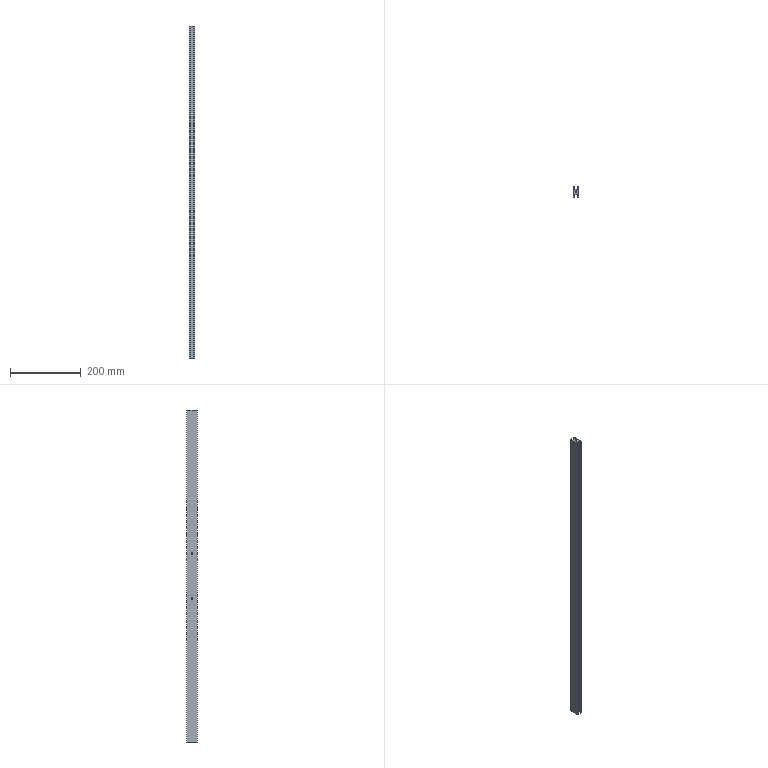Part | SolidWorks | features BaseBody 1 | 1 solid | 40 faces | box 15 x 30 x 936 mm | volume 263254 mm3 | plane 30 | cylinder 10 | commonest cylinder face diameters 4.2 x8 5 x2